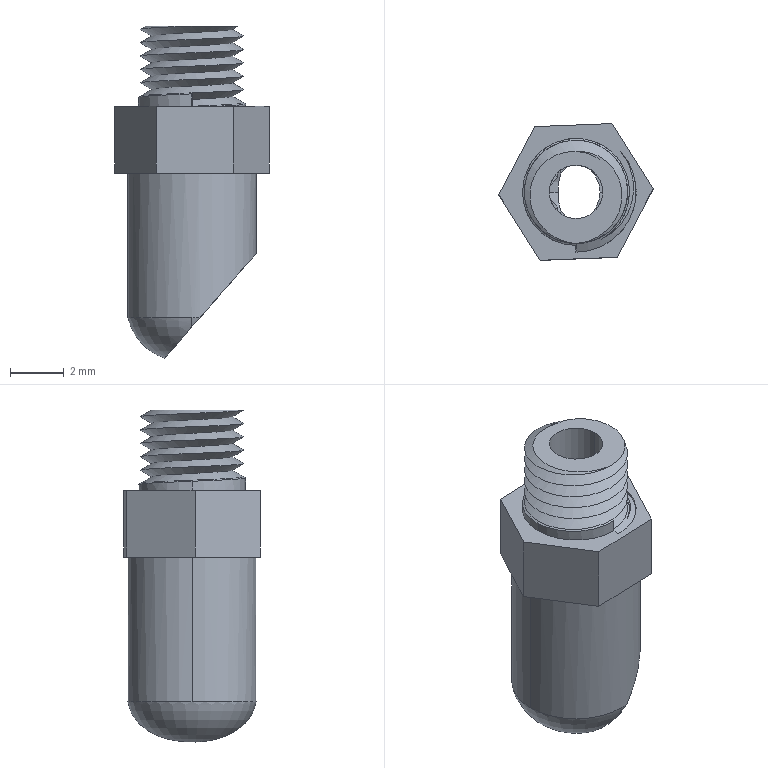Part | SolidWorks | features BaseBody 1 | 1 solid | 39 faces | box 5.769 x 5.109 x 12.413 mm | volume 137.319 mm3 | plane 17 | cylinder 12 | cone 4 | torus 3 | spline 3 | commonest cylinder face diameters 2 x4 4 x3 3.3 x2 4.8 x2 4.5 x1